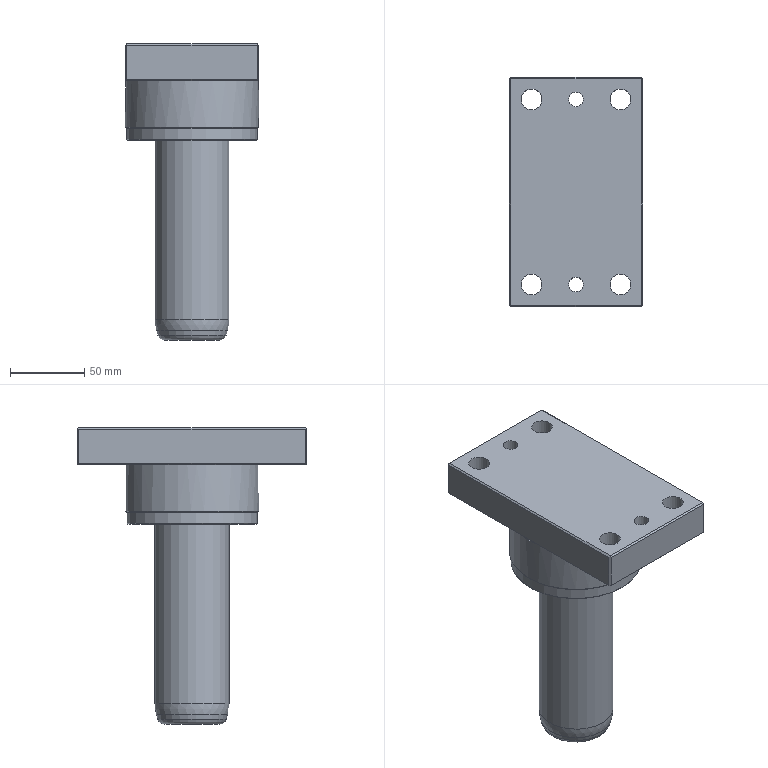Part | NX | features solid 2 | 1 solid | 46 faces | box 90 x 155 x 200 mm | volume 838352 mm3 | plane 26 | cylinder 13 | cone 5 | torus 2 | commonest cylinder face diameters 14 x4 50 x3 10 x2 12 x1 46 x1 88 x1
STEP:
#1=CARTESIAN_POINT('',(360.,263.5,441.));
#2=VERTEX_POINT('',#1);
#3=CARTESIAN_POINT('',(360.,334.084,441.));
#4=VERTEX_POINT('',#3);
#5=CARTESIAN_POINT('',(360.,262.5,441.));
#6=DIRECTION('',(0.,1.,0.));
#7=VECTOR('',#6,1000.);
#8=LINE('',#5,#7);
#9=EDGE_CURVE('',#2,#4,#8,.T.);
#10=ORIENTED_EDGE('',*,*,#9,.T.);
#11=CARTESIAN_POINT('',(360.,345.916,441.));
#12=VERTEX_POINT('',#11);
#13=CARTESIAN_POINT('',(360.,340.,440.));
#14=DIRECTION('',(1.,0.,0.));
#15=DIRECTION('',(0.,-1.,0.));
#16=AXIS2_PLACEMENT_3D('',#13,#14,#15);
#17=CIRCLE('',#16,6.);
#18=EDGE_CURVE('',#12,#4,#17,.T.);
#19=ORIENTED_EDGE('',*,*,#18,.F.);
#20=CARTESIAN_POINT('',(360.,416.5,441.));
#21=VERTEX_POINT('',#20);
#22=CARTESIAN_POINT('',(360.,262.5,441.));
#23=DIRECTION('',(0.,1.,0.));
#24=VECTOR('',#23,1000.);
#25=LINE('',#22,#24);
#26=EDGE_CURVE('',#12,#21,#25,.T.);
#27=ORIENTED_EDGE('',*,*,#26,.T.);
#28=CARTESIAN_POINT('',(360.,416.5,464.));
#29=VERTEX_POINT('',#28);
#30=CARTESIAN_POINT('',(360.,416.5,440.));
#31=DIRECTION('',(0.,0.,1.));
#32=VECTOR('',#31,1000.);
#33=LINE('',#30,#32);
#34=EDGE_CURVE('',#21,#29,#33,.T.);
#35=ORIENTED_EDGE('',*,*,#34,.T.);
#36=CARTESIAN_POINT('',(360.,263.5,464.));
#37=VERTEX_POINT('',#36);
#38=CARTESIAN_POINT('',(360.,262.5,464.));
#39=DIRECTION('',(0.,-1.,0.));
#40=VECTOR('',#39,1000.);
#41=LINE('',#38,#40);
#42=EDGE_CURVE('',#29,#37,#41,.T.);
#43=ORIENTED_EDGE('',*,*,#42,.T.);
#44=CARTESIAN_POINT('',(360.,263.5,440.));
#45=DIRECTION('',(0.,0.,-1.));
#46=VECTOR('',#45,1000.);
#47=LINE('',#44,#46);
#48=EDGE_CURVE('',#37,#2,#47,.T.);
#49=ORIENTED_EDGE('',*,*,#48,.T.);
#50=EDGE_LOOP('',(#10,#19,#27,#35,#43,#49));
#51=FACE_BOUND('',#50,.T.);
#52=CARTESIAN_POINT('',(360.,262.5,440.));
#53=DIRECTION('',(1.,0.,0.));
#54=DIRECTION('',(0.,-1.,0.));
#55=AXIS2_PLACEMENT_3D('',#52,#53,#54);
#56=PLANE('',#55);
#57=ADVANCED_FACE('',(#51),#56,.T.);
#58=CARTESIAN_POINT('',(359.,334.,440.));
#59=VERTEX_POINT('',#58);
#60=CARTESIAN_POINT('',(359.,330.566,440.));
#61=VERTEX_POINT('',#60);
#62=CARTESIAN_POINT('',(359.,417.5,440.));
#63=DIRECTION('',(0.,-1.,0.));
#64=VECTOR('',#63,1000.);
#65=LINE('',#62,#64);
#66=EDGE_CURVE('',#59,#61,#65,.T.);
#67=ORIENTED_EDGE('',*,*,#66,.F.);
#68=CARTESIAN_POINT('',(359.,340.,440.));
#69=DIRECTION('',(-0.7071,0.,0.7071));
#70=DIRECTION('',(-0.7071,0.,-0.7071));
#71=AXIS2_PLACEMENT_3D('',#68,#69,#70);
#72=ELLIPSE('',#71,8.485,6.);
#73=EDGE_CURVE('',#59,#4,#72,.T.);
#74=ORIENTED_EDGE('',*,*,#73,.T.);
#75=ORIENTED_EDGE('',*,*,#9,.F.);
#76=CARTESIAN_POINT('',(359.5,263.,440.5));
#77=VERTEX_POINT('',#76);
#78=CARTESIAN_POINT('',(359.667,263.167,440.667));
#79=DIRECTION('',(-0.5774,-0.5774,-0.5774));
#80=VECTOR('',#79,1000.);
#81=LINE('',#78,#80);
#82=EDGE_CURVE('',#2,#77,#81,.T.);
#83=ORIENTED_EDGE('',*,*,#82,.T.);
#84=CARTESIAN_POINT('',(359.,263.5,440.));
#85=VERTEX_POINT('',#84);
#86=CARTESIAN_POINT('',(360.,262.5,441.));
#87=DIRECTION('',(-0.5774,0.5774,-0.5774));
#88=VECTOR('',#87,1000.);
#89=LINE('',#86,#88);
#90=EDGE_CURVE('',#85,#77,#89,.F.);
#91=ORIENTED_EDGE('',*,*,#90,.F.);
#92=CARTESIAN_POINT('',(359.,417.5,440.));
#93=DIRECTION('',(0.,-1.,0.));
#94=VECTOR('',#93,1000.);
#95=LINE('',#92,#94);
#96=EDGE_CURVE('',#61,#85,#95,.T.);
#97=ORIENTED_EDGE('',*,*,#96,.F.);
#98=EDGE_LOOP('',(#67,#74,#75,#83,#91,#97));
#99=FACE_BOUND('',#98,.T.);
#100=CARTESIAN_POINT('',(360.,262.5,441.));
#101=DIRECTION('',(-0.7071,0.,0.7071));
#102=DIRECTION('',(-0.7071,0.,-0.7071));
#103=AXIS2_PLACEMENT_3D('',#100,#101,#102);
#104=PLANE('',#103);
#105=ADVANCED_FACE('',(#99),#104,.F.);
#106=ORIENTED_EDGE('',*,*,#26,.F.);
#107=CARTESIAN_POINT('',(359.,346.,440.));
#108=VERTEX_POINT('',#107);
#109=CARTESIAN_POINT('',(359.,340.,440.));
#110=DIRECTION('',(-0.7071,0.,0.7071));
#111=DIRECTION('',(-0.7071,0.,-0.7071));
#112=AXIS2_PLACEMENT_3D('',#109,#110,#111);
#113=ELLIPSE('',#112,8.485,6.);
#114=EDGE_CURVE('',#12,#108,#113,.T.);
#115=ORIENTED_EDGE('',*,*,#114,.T.);
#116=CARTESIAN_POINT('',(359.,349.434,440.));
#117=VERTEX_POINT('',#116);
#118=CARTESIAN_POINT('',(359.,417.5,440.));
#119=DIRECTION('',(0.,-1.,0.));
#120=VECTOR('',#119,1000.);
#121=LINE('',#118,#120);
#122=EDGE_CURVE('',#117,#108,#121,.T.);
#123=ORIENTED_EDGE('',*,*,#122,.F.);
#124=CARTESIAN_POINT('',(359.,416.5,440.));
#125=VERTEX_POINT('',#124);
#126=CARTESIAN_POINT('',(359.,417.5,440.));
#127=DIRECTION('',(0.,-1.,0.));
#128=VECTOR('',#127,1000.);
#129=LINE('',#126,#128);
#130=EDGE_CURVE('',#125,#117,#129,.T.);
#131=ORIENTED_EDGE('',*,*,#130,.F.);
#132=CARTESIAN_POINT('',(359.5,417.,440.5));
#133=VERTEX_POINT('',#132);
#134=CARTESIAN_POINT('',(360.,417.5,441.));
#135=DIRECTION('',(-0.5774,-0.5774,-0.5774));
#136=VECTOR('',#135,1000.);
#137=LINE('',#134,#136);
#138=EDGE_CURVE('',#125,#133,#137,.F.);
#139=ORIENTED_EDGE('',*,*,#138,.T.);
#140=CARTESIAN_POINT('',(411.333,365.167,492.333));
#141=DIRECTION('',(0.5774,-0.5774,0.5774));
#142=VECTOR('',#141,1000.);
#143=LINE('',#140,#142);
#144=EDGE_CURVE('',#133,#21,#143,.T.);
#145=ORIENTED_EDGE('',*,*,#144,.T.);
#146=EDGE_LOOP('',(#106,#115,#123,#131,#139,#145));
#147=FACE_BOUND('',#146,.T.);
#148=CARTESIAN_POINT('',(360.,262.5,441.));
#149=DIRECTION('',(-0.7071,0.,0.7071));
#150=DIRECTION('',(-0.7071,0.,-0.7071));
#151=AXIS2_PLACEMENT_3D('',#148,#149,#150);
#152=PLANE('',#151);
#153=ADVANCED_FACE('',(#147),#152,.F.);
#154=CARTESIAN_POINT('',(359.598,334.,440.));
#155=VERTEX_POINT('',#154);
#156=CARTESIAN_POINT('',(360.,334.,440.));
#157=DIRECTION('',(-1.,0.,0.));
#158=VECTOR('',#157,1000.);
#159=LINE('',#156,#158);
#160=EDGE_CURVE('',#59,#155,#159,.F.);
#161=ORIENTED_EDGE('',*,*,#160,.F.);
#162=ORIENTED_EDGE('',*,*,#66,.T.);
#163=CARTESIAN_POINT('',(315.,340.,440.));
#164=DIRECTION('',(0.,0.,-1.));
#165=DIRECTION('',(0.,-1.,0.));
#166=AXIS2_PLACEMENT_3D('',#163,#164,#165);
#167=CIRCLE('',#166,45.);
#168=EDGE_CURVE('',#155,#61,#167,.T.);
#169=ORIENTED_EDGE('',*,*,#168,.F.);
#170=EDGE_LOOP('',(#161,#162,#169));
#171=FACE_BOUND('',#170,.T.);
#172=CARTESIAN_POINT('',(315.,340.,440.));
#173=DIRECTION('',(0.,0.,-1.));
#174=DIRECTION('',(0.,-1.,0.));
#175=AXIS2_PLACEMENT_3D('',#172,#173,#174);
#176=PLANE('',#175);
#177=ADVANCED_FACE('',(#171),#176,.F.);
#178=CARTESIAN_POINT('',(359.598,346.,440.));
#179=VERTEX_POINT('',#178);
#180=CARTESIAN_POINT('',(360.,346.,440.));
#181=DIRECTION('',(-1.,0.,0.));
#182=VECTOR('',#181,1000.);
#183=LINE('',#180,#182);
#184=EDGE_CURVE('',#179,#108,#183,.T.);
#185=ORIENTED_EDGE('',*,*,#184,.F.);
#186=CARTESIAN_POINT('',(315.,340.,440.));
#187=DIRECTION('',(0.,0.,-1.));
#188=DIRECTION('',(0.,-1.,0.));
#189=AXIS2_PLACEMENT_3D('',#186,#187,#188);
#190=CIRCLE('',#189,45.);
#191=EDGE_CURVE('',#117,#179,#190,.T.);
#192=ORIENTED_EDGE('',*,*,#191,.F.);
#193=ORIENTED_EDGE('',*,*,#122,.T.);
#194=EDGE_LOOP('',(#185,#192,#193));
#195=FACE_BOUND('',#194,.T.);
#196=CARTESIAN_POINT('',(315.,340.,440.));
#197=DIRECTION('',(0.,0.,-1.));
#198=DIRECTION('',(0.,-1.,0.));
#199=AXIS2_PLACEMENT_3D('',#196,#197,#198);
#200=PLANE('',#199);
#201=ADVANCED_FACE('',(#195),#200,.F.);
#202=CARTESIAN_POINT('',(315.,295.,408.625));
#203=VERTEX_POINT('',#202);
#204=CARTESIAN_POINT('',(315.,340.,408.625));
#205=DIRECTION('',(0.,0.,-1.));
#206=DIRECTION('',(0.,-1.,0.));
#207=AXIS2_PLACEMENT_3D('',#204,#205,#206);
#208=CIRCLE('',#207,45.);
#209=EDGE_CURVE('',#203,#203,#208,.F.);
#210=ORIENTED_EDGE('',*,*,#209,.T.);
#211=EDGE_LOOP('',(#210));
#212=FACE_BOUND('',#211,.T.);
#213=CARTESIAN_POINT('',(359.598,334.,440.));
#214=CARTESIAN_POINT('',(359.598,334.,438.413));
#215=CARTESIAN_POINT('',(359.8,335.296,435.31));
#216=CARTESIAN_POINT('',(360.1,340.001,433.346));
#217=CARTESIAN_POINT('',(359.8,344.699,435.306));
#218=CARTESIAN_POINT('',(359.598,346.,438.413));
#219=CARTESIAN_POINT('',(359.598,346.,440.));
#220=B_SPLINE_CURVE_WITH_KNOTS('',3,(#213,#214,#215,#216,#217,#218,#219),.UNSPECIFIED.,.F.,.F.,(4,1,1,1,4),(0.,0.004692,0.009383,0.01408,0.01877),.UNSPECIFIED.);
#221=EDGE_CURVE('',#155,#179,#220,.T.);
#222=ORIENTED_EDGE('',*,*,#221,.F.);
#223=ORIENTED_EDGE('',*,*,#168,.T.);
#224=CARTESIAN_POINT('',(271.,330.566,440.));
#225=VERTEX_POINT('',#224);
#226=CARTESIAN_POINT('',(315.,340.,440.));
#227=DIRECTION('',(0.,0.,-1.));
#228=DIRECTION('',(0.,-1.,0.));
#229=AXIS2_PLACEMENT_3D('',#226,#227,#228);
#230=CIRCLE('',#229,45.);
#231=EDGE_CURVE('',#61,#225,#230,.T.);
#232=ORIENTED_EDGE('',*,*,#231,.T.);
#233=CARTESIAN_POINT('',(271.,349.434,440.));
#234=VERTEX_POINT('',#233);
#235=CARTESIAN_POINT('',(315.,340.,440.));
#236=DIRECTION('',(0.,0.,-1.));
#237=DIRECTION('',(0.,-1.,0.));
#238=AXIS2_PLACEMENT_3D('',#235,#236,#237);
#239=CIRCLE('',#238,45.);
#240=EDGE_CURVE('',#225,#234,#239,.T.);
#241=ORIENTED_EDGE('',*,*,#240,.T.);
#242=CARTESIAN_POINT('',(315.,340.,440.));
#243=DIRECTION('',(0.,0.,-1.));
#244=DIRECTION('',(0.,-1.,0.));
#245=AXIS2_PLACEMENT_3D('',#242,#243,#244);
#246=CIRCLE('',#245,45.);
#247=EDGE_CURVE('',#234,#117,#246,.T.);
#248=ORIENTED_EDGE('',*,*,#247,.T.);
#249=ORIENTED_EDGE('',*,*,#191,.T.);
#250=EDGE_LOOP('',(#222,#223,#232,#241,#248,#249));
#251=FACE_BOUND('',#250,.T.);
#252=CARTESIAN_POINT('',(315.,340.,408.125));
#253=DIRECTION('',(0.,0.,1.));
#254=DIRECTION('',(0.,1.,0.));
#255=AXIS2_PLACEMENT_3D('',#252,#253,#254);
#256=CYLINDRICAL_SURFACE('',#255,45.);
#257=ADVANCED_FACE('',(#212,#251),#256,.T.);
#258=CARTESIAN_POINT('',(315.,365.,426.5));
#259=VERTEX_POINT('',#258);
#260=CARTESIAN_POINT('',(315.,340.,426.5));
#261=DIRECTION('',(0.,0.,-1.));
#262=DIRECTION('',(0.,1.,0.));
#263=AXIS2_PLACEMENT_3D('',#260,#261,#262);
#264=CIRCLE('',#263,25.);
#265=EDGE_CURVE('',#259,#259,#264,.F.);
#266=ORIENTED_EDGE('',*,*,#265,.F.);
#267=EDGE_LOOP('',(#266));
#268=FACE_BOUND('',#267,.T.);
#269=CARTESIAN_POINT('',(339.316,345.809,438.5));
#270=VERTEX_POINT('',#269);
#271=CARTESIAN_POINT('',(339.316,334.191,438.5));
#272=VERTEX_POINT('',#271);
#273=CARTESIAN_POINT('',(315.,340.,438.5));
#274=DIRECTION('',(0.,0.,-1.));
#275=DIRECTION('',(0.,-1.,0.));
#276=AXIS2_PLACEMENT_3D('',#273,#274,#275);
#277=CIRCLE('',#276,25.);
#278=EDGE_CURVE('',#270,#272,#277,.F.);
#279=ORIENTED_EDGE('',*,*,#278,.T.);
#280=CARTESIAN_POINT('',(339.316,334.191,438.5));
#281=CARTESIAN_POINT('',(339.395,334.522,437.217));
#282=CARTESIAN_POINT('',(339.758,336.04,434.912));
#283=CARTESIAN_POINT('',(340.121,340.007,433.543));
#284=CARTESIAN_POINT('',(339.758,343.961,434.917));
#285=CARTESIAN_POINT('',(339.395,345.477,437.213));
#286=CARTESIAN_POINT('',(339.316,345.809,438.5));
#287=B_SPLINE_CURVE_WITH_KNOTS('',3,(#280,#281,#282,#283,#284,#285,#286),.UNSPECIFIED.,.F.,.F.,(4,1,1,1,4),(0.02975,0.0337,0.03765,0.04161,0.04556),.UNSPECIFIED.);
#288=EDGE_CURVE('',#272,#270,#287,.T.);
#289=ORIENTED_EDGE('',*,*,#288,.T.);
#290=EDGE_LOOP('',(#279,#289));
#291=FACE_BOUND('',#290,.T.);
#292=CARTESIAN_POINT('',(315.,340.,400.));
#293=DIRECTION('',(0.,0.,1.));
#294=DIRECTION('',(0.,1.,0.));
#295=AXIS2_PLACEMENT_3D('',#292,#293,#294);
#296=CYLINDRICAL_SURFACE('',#295,25.);
#297=ADVANCED_FACE('',(#268,#291),#296,.F.);
#298=CARTESIAN_POINT('',(315.,407.5,465.));
#299=VERTEX_POINT('',#298);
#300=CARTESIAN_POINT('',(315.,402.5,465.));
#301=DIRECTION('',(0.,0.,1.));
#302=DIRECTION('',(0.,1.,0.));
#303=AXIS2_PLACEMENT_3D('',#300,#301,#302);
#304=CIRCLE('',#303,5.);
#305=EDGE_CURVE('',#299,#299,#304,.T.);
#306=ORIENTED_EDGE('',*,*,#305,.F.);
#307=EDGE_LOOP('',(#306));
#308=FACE_BOUND('',#307,.T.);
#309=CARTESIAN_POINT('',(345.,409.5,465.));
#310=VERTEX_POINT('',#309);
#311=CARTESIAN_POINT('',(345.,402.5,465.));
#312=DIRECTION('',(0.,0.,-1.));
#313=DIRECTION('',(0.,1.,0.));
#314=AXIS2_PLACEMENT_3D('',#311,#312,#313);
#315=CIRCLE('',#314,7.);
#316=EDGE_CURVE('',#310,#310,#315,.T.);
#317=ORIENTED_EDGE('',*,*,#316,.T.);
#318=EDGE_LOOP('',(#317));
#319=FACE_BOUND('',#318,.T.);
#320=CARTESIAN_POINT('',(345.,270.5,465.));
#321=VERTEX_POINT('',#320);
#322=CARTESIAN_POINT('',(345.,277.5,465.));
#323=DIRECTION('',(0.,0.,1.));
#324=DIRECTION('',(0.,-1.,0.));
#325=AXIS2_PLACEMENT_3D('',#322,#323,#324);
#326=CIRCLE('',#325,7.);
#327=EDGE_CURVE('',#321,#321,#326,.T.);
#328=ORIENTED_EDGE('',*,*,#327,.F.);
#329=EDGE_LOOP('',(#328));
#330=FACE_BOUND('',#329,.T.);
#331=CARTESIAN_POINT('',(271.,416.5,465.));
#332=VERTEX_POINT('',#331);
#333=CARTESIAN_POINT('',(271.,263.5,465.));
#334=VERTEX_POINT('',#333);
#335=CARTESIAN_POINT('',(271.,262.5,465.));
#336=DIRECTION('',(0.,-1.,0.));
#337=VECTOR('',#336,1000.);
#338=LINE('',#335,#337);
#339=EDGE_CURVE('',#332,#334,#338,.T.);
#340=ORIENTED_EDGE('',*,*,#339,.T.);
#341=CARTESIAN_POINT('',(359.,263.5,465.));
#342=VERTEX_POINT('',#341);
#343=CARTESIAN_POINT('',(360.,263.5,465.));
#344=DIRECTION('',(1.,0.,0.));
#345=VECTOR('',#344,1000.);
#346=LINE('',#343,#345);
#347=EDGE_CURVE('',#334,#342,#346,.T.);
#348=ORIENTED_EDGE('',*,*,#347,.T.);
#349=CARTESIAN_POINT('',(359.,416.5,465.));
#350=VERTEX_POINT('',#349);
#351=CARTESIAN_POINT('',(359.,417.5,465.));
#352=DIRECTION('',(0.,1.,0.));
#353=VECTOR('',#352,1000.);
#354=LINE('',#351,#353);
#355=EDGE_CURVE('',#342,#350,#354,.T.);
#356=ORIENTED_EDGE('',*,*,#355,.T.);
#357=CARTESIAN_POINT('',(270.,416.5,465.));
#358=DIRECTION('',(-1.,0.,0.));
#359=VECTOR('',#358,1000.);
#360=LINE('',#357,#359);
#361=EDGE_CURVE('',#350,#332,#360,.T.);
#362=ORIENTED_EDGE('',*,*,#361,.T.);
#363=EDGE_LOOP('',(#340,#348,#356,#362));
#364=FACE_BOUND('',#363,.T.);
#365=CARTESIAN_POINT('',(285.,270.5,465.));
#366=VERTEX_POINT('',#365);
#367=CARTESIAN_POINT('',(285.,277.5,465.));
#368=DIRECTION('',(0.,0.,-1.));
#369=DIRECTION('',(0.,-1.,0.));
#370=AXIS2_PLACEMENT_3D('',#367,#368,#369);
#371=CIRCLE('',#370,7.);
#372=EDGE_CURVE('',#366,#366,#371,.T.);
#373=ORIENTED_EDGE('',*,*,#372,.T.);
#374=EDGE_LOOP('',(#373));
#375=FACE_BOUND('',#374,.T.);
#376=CARTESIAN_POINT('',(285.,409.5,465.));
#377=VERTEX_POINT('',#376);
#378=CARTESIAN_POINT('',(285.,402.5,465.));
#379=DIRECTION('',(0.,0.,1.));
#380=DIRECTION('',(0.,1.,0.));
#381=AXIS2_PLACEMENT_3D('',#378,#379,#380);
#382=CIRCLE('',#381,7.);
#383=EDGE_CURVE('',#377,#377,#382,.T.);
#384=ORIENTED_EDGE('',*,*,#383,.F.);
#385=EDGE_LOOP('',(#384));
#386=FACE_BOUND('',#385,.T.);
#387=CARTESIAN_POINT('',(315.,272.5,465.));
#388=VERTEX_POINT('',#387);
#389=CARTESIAN_POINT('',(315.,277.5,465.));
#390=DIRECTION('',(0.,0.,-1.));
#391=DIRECTION('',(0.,-1.,0.));
#392=AXIS2_PLACEMENT_3D('',#389,#390,#391);
#393=CIRCLE('',#392,5.);
#394=EDGE_CURVE('',#388,#388,#393,.T.);
#395=ORIENTED_EDGE('',*,*,#394,.T.);
#396=EDGE_LOOP('',(#395));
#397=FACE_BOUND('',#396,.T.);
#398=CARTESIAN_POINT('',(360.,417.5,465.));
#399=DIRECTION('',(0.,0.,-1.));
#400=DIRECTION('',(0.,-1.,0.));
#401=AXIS2_PLACEMENT_3D('',#398,#399,#400);
#402=PLANE('',#401);
#403=ADVANCED_FACE('',(#308,#319,#330,#364,#375,#386,#397),#402,.F.);
#404=CARTESIAN_POINT('',(285.,270.5,440.));
#405=VERTEX_POINT('',#404);
#406=CARTESIAN_POINT('',(285.,277.5,440.));
#407=DIRECTION('',(0.,0.,-1.));
#408=DIRECTION('',(0.,-1.,0.));
#409=AXIS2_PLACEMENT_3D('',#406,#407,#408);
#410=CIRCLE('',#409,7.);
#411=EDGE_CURVE('',#405,#405,#410,.F.);
#412=ORIENTED_EDGE('',*,*,#411,.T.);
#413=EDGE_LOOP('',(#412));
#414=FACE_BOUND('',#413,.T.);
#415=ORIENTED_EDGE('',*,*,#231,.F.);
#416=ORIENTED_EDGE('',*,*,#96,.T.);
#417=CARTESIAN_POINT('',(271.,263.5,440.));
#418=VERTEX_POINT('',#417);
#419=CARTESIAN_POINT('',(360.,263.5,440.));
#420=DIRECTION('',(-1.,0.,0.));
#421=VECTOR('',#420,1000.);
#422=LINE('',#419,#421);
#423=EDGE_CURVE('',#85,#418,#422,.T.);
#424=ORIENTED_EDGE('',*,*,#423,.T.);
#425=CARTESIAN_POINT('',(271.,417.5,440.));
#426=DIRECTION('',(0.,1.,0.));
#427=VECTOR('',#426,1000.);
#428=LINE('',#425,#427);
#429=EDGE_CURVE('',#418,#225,#428,.T.);
#430=ORIENTED_EDGE('',*,*,#429,.T.);
#431=EDGE_LOOP('',(#415,#416,#424,#430));
#432=FACE_BOUND('',#431,.T.);
#433=CARTESIAN_POINT('',(345.,270.5,440.));
#434=VERTEX_POINT('',#433);
#435=CARTESIAN_POINT('',(345.,277.5,440.));
#436=DIRECTION('',(0.,0.,-1.));
#437=DIRECTION('',(0.,-1.,0.));
#438=AXIS2_PLACEMENT_3D('',#435,#436,#437);
#439=CIRCLE('',#438,7.);
#440=EDGE_CURVE('',#434,#434,#439,.T.);
#441=ORIENTED_EDGE('',*,*,#440,.F.);
#442=EDGE_LOOP('',(#441));
#443=FACE_BOUND('',#442,.T.);
#444=CARTESIAN_POINT('',(315.,272.5,440.));
#445=VERTEX_POINT('',#444);
#446=CARTESIAN_POINT('',(315.,277.5,440.));
#447=DIRECTION('',(0.,0.,-1.));
#448=DIRECTION('',(0.,-1.,0.));
#449=AXIS2_PLACEMENT_3D('',#446,#447,#448);
#450=CIRCLE('',#449,5.);
#451=EDGE_CURVE('',#445,#445,#450,.T.);
#452=ORIENTED_EDGE('',*,*,#451,.F.);
#453=EDGE_LOOP('',(#452));
#454=FACE_BOUND('',#453,.T.);
#455=CARTESIAN_POINT('',(360.,417.5,440.));
#456=DIRECTION('',(0.,0.,-1.));
#457=DIRECTION('',(0.,-1.,0.));
#458=AXIS2_PLACEMENT_3D('',#455,#456,#457);
#459=PLANE('',#458);
#460=ADVANCED_FACE('',(#414,#432,#443,#454),#459,.T.);
#461=CARTESIAN_POINT('',(315.,407.5,440.));
#462=VERTEX_POINT('',#461);
#463=CARTESIAN_POINT('',(315.,402.5,440.));
#464=DIRECTION('',(0.,0.,1.));
#465=DIRECTION('',(0.,1.,0.));
#466=AXIS2_PLACEMENT_3D('',#463,#464,#465);
#467=CIRCLE('',#466,5.);
#468=EDGE_CURVE('',#462,#462,#467,.T.);
#469=ORIENTED_EDGE('',*,*,#468,.T.);
#470=EDGE_LOOP('',(#469));
#471=FACE_BOUND('',#470,.T.);
#472=CARTESIAN_POINT('',(285.,395.5,440.));
#473=VERTEX_POINT('',#472);
#474=CARTESIAN_POINT('',(285.,402.5,440.));
#475=DIRECTION('',(0.,0.,-1.));
#476=DIRECTION('',(0.,-1.,0.));
#477=AXIS2_PLACEMENT_3D('',#474,#475,#476);
#478=CIRCLE('',#477,7.);
#479=EDGE_CURVE('',#473,#473,#478,.T.);
#480=ORIENTED_EDGE('',*,*,#479,.F.);
#481=EDGE_LOOP('',(#480));
#482=FACE_BOUND('',#481,.T.);
#483=ORIENTED_EDGE('',*,*,#247,.F.);
#484=CARTESIAN_POINT('',(271.,416.5,440.));
#485=VERTEX_POINT('',#484);
#486=CARTESIAN_POINT('',(271.,417.5,440.));
#487=DIRECTION('',(0.,1.,0.));
#488=VECTOR('',#487,1000.);
#489=LINE('',#486,#488);
#490=EDGE_CURVE('',#234,#485,#489,.T.);
#491=ORIENTED_EDGE('',*,*,#490,.T.);
#492=CARTESIAN_POINT('',(360.,416.5,440.));
#493=DIRECTION('',(1.,0.,0.));
#494=VECTOR('',#493,1000.);
#495=LINE('',#492,#494);
#496=EDGE_CURVE('',#485,#125,#495,.T.);
#497=ORIENTED_EDGE('',*,*,#496,.T.);
#498=ORIENTED_EDGE('',*,*,#130,.T.);
#499=EDGE_LOOP('',(#483,#491,#497,#498));
#500=FACE_BOUND('',#499,.T.);
#501=CARTESIAN_POINT('',(345.,395.5,440.));
#502=VERTEX_POINT('',#501);
#503=CARTESIAN_POINT('',(345.,402.5,440.));
#504=DIRECTION('',(0.,0.,-1.));
#505=DIRECTION('',(0.,-1.,0.));
#506=AXIS2_PLACEMENT_3D('',#503,#504,#505);
#507=CIRCLE('',#506,7.);
#508=EDGE_CURVE('',#502,#502,#507,.F.);
#509=ORIENTED_EDGE('',*,*,#508,.T.);
#510=EDGE_LOOP('',(#509));
#511=FACE_BOUND('',#510,.T.);
#512=CARTESIAN_POINT('',(360.,417.5,440.));
#513=DIRECTION('',(0.,0.,-1.));
#514=DIRECTION('',(0.,-1.,0.));
#515=AXIS2_PLACEMENT_3D('',#512,#513,#514);
#516=PLANE('',#515);
#517=ADVANCED_FACE('',(#471,#482,#500,#511),#516,.T.);
#518=CARTESIAN_POINT('',(315.,296.5,400.));
#519=VERTEX_POINT('',#518);
#520=CARTESIAN_POINT('',(315.,340.,400.));
#521=DIRECTION('',(0.,0.,-1.));
#522=DIRECTION('',(0.,-1.,0.));
#523=AXIS2_PLACEMENT_3D('',#520,#521,#522);
#524=CIRCLE('',#523,43.5);
#525=EDGE_CURVE('',#519,#519,#524,.T.);
#526=ORIENTED_EDGE('',*,*,#525,.T.);
#527=EDGE_LOOP('',(#526));
#528=FACE_BOUND('',#527,.T.);
#529=CARTESIAN_POINT('',(315.,315.,400.));
#530=VERTEX_POINT('',#529);
#531=CARTESIAN_POINT('',(315.,340.,400.));
#532=DIRECTION('',(0.,0.,-1.));
#533=DIRECTION('',(0.,-1.,0.));
#534=AXIS2_PLACEMENT_3D('',#531,#532,#533);
#535=CIRCLE('',#534,25.);
#536=EDGE_CURVE('',#530,#530,#535,.T.);
#537=ORIENTED_EDGE('',*,*,#536,.F.);
#538=EDGE_LOOP('',(#537));
#539=FACE_BOUND('',#538,.T.);
#540=CARTESIAN_POINT('',(315.,340.,400.));
#541=DIRECTION('',(0.,0.,-1.));
#542=DIRECTION('',(0.,-1.,0.));
#543=AXIS2_PLACEMENT_3D('',#540,#541,#542);
#544=PLANE('',#543);
#545=ADVANCED_FACE('',(#528,#539),#544,.T.);
#546=CARTESIAN_POINT('',(315.,295.5,408.125));
#547=VERTEX_POINT('',#546);
#548=CARTESIAN_POINT('',(315.,340.,408.125));
#549=DIRECTION('',(0.,0.,-1.));
#550=DIRECTION('',(0.,-1.,0.));
#551=AXIS2_PLACEMENT_3D('',#548,#549,#550);
#552=CIRCLE('',#551,44.5);
#553=EDGE_CURVE('',#547,#547,#552,.T.);
#554=ORIENTED_EDGE('',*,*,#553,.T.);
#555=EDGE_LOOP('',(#554));
#556=FACE_BOUND('',#555,.T.);
#557=CARTESIAN_POINT('',(315.,296.,408.125));
#558=VERTEX_POINT('',#557);
#559=CARTESIAN_POINT('',(315.,340.,408.125));
#560=DIRECTION('',(0.,0.,-1.));
#561=DIRECTION('',(0.,-1.,0.));
#562=AXIS2_PLACEMENT_3D('',#559,#560,#561);
#563=CIRCLE('',#562,44.);
#564=EDGE_CURVE('',#558,#558,#563,.T.);
#565=ORIENTED_EDGE('',*,*,#564,.F.);
#566=EDGE_LOOP('',(#565));
#567=FACE_BOUND('',#566,.T.);
#568=CARTESIAN_POINT('',(315.,340.,408.125));
#569=DIRECTION('',(0.,0.,-1.));
#570=DIRECTION('',(0.,-1.,0.));
#571=AXIS2_PLACEMENT_3D('',#568,#569,#570);
#572=PLANE('',#571);
#573=ADVANCED_FACE('',(#556,#567),#572,.T.);
#574=CARTESIAN_POINT('',(271.,417.5,464.));
#575=VERTEX_POINT('',#574);
#576=CARTESIAN_POINT('',(359.,417.5,464.));
#577=VERTEX_POINT('',#576);
#578=CARTESIAN_POINT('',(360.,417.5,464.));
#579=DIRECTION('',(1.,0.,0.));
#580=VECTOR('',#579,1000.);
#581=LINE('',#578,#580);
#582=EDGE_CURVE('',#575,#577,#581,.T.);
#583=ORIENTED_EDGE('',*,*,#582,.T.);
#584=CARTESIAN_POINT('',(359.,417.5,441.));
#585=VERTEX_POINT('',#584);
#586=CARTESIAN_POINT('',(359.,417.5,440.));
#587=DIRECTION('',(0.,0.,-1.));
#588=VECTOR('',#587,1000.);
#589=LINE('',#586,#588);
#590=EDGE_CURVE('',#577,#585,#589,.T.);
#591=ORIENTED_EDGE('',*,*,#590,.T.);
#592=CARTESIAN_POINT('',(271.,417.5,441.));
#593=VERTEX_POINT('',#592);
#594=CARTESIAN_POINT('',(360.,417.5,441.));
#595=DIRECTION('',(-1.,0.,0.));
#596=VECTOR('',#595,1000.);
#597=LINE('',#594,#596);
#598=EDGE_CURVE('',#585,#593,#597,.T.);
#599=ORIENTED_EDGE('',*,*,#598,.T.);
#600=CARTESIAN_POINT('',(271.,417.5,440.));
#601=DIRECTION('',(0.,0.,1.));
#602=VECTOR('',#601,1000.);
#603=LINE('',#600,#602);
#604=EDGE_CURVE('',#593,#575,#603,.T.);
#605=ORIENTED_EDGE('',*,*,#604,.T.);
#606=EDGE_LOOP('',(#583,#591,#599,#605));
#607=FACE_BOUND('',#606,.T.);
#608=CARTESIAN_POINT('',(360.,417.5,440.));
#609=DIRECTION('',(0.,1.,0.));
#610=DIRECTION('',(0.,0.,-1.));
#611=AXIS2_PLACEMENT_3D('',#608,#609,#610);
#612=PLANE('',#611);
#613=ADVANCED_FACE('',(#607),#612,.T.);
#614=CARTESIAN_POINT('',(270.,263.5,464.));
#615=VERTEX_POINT('',#614);
#616=CARTESIAN_POINT('',(270.,416.5,464.));
#617=VERTEX_POINT('',#616);
#618=CARTESIAN_POINT('',(270.,417.5,464.));
#619=DIRECTION('',(0.,1.,0.));
#620=VECTOR('',#619,1000.);
#621=LINE('',#618,#620);
#622=EDGE_CURVE('',#615,#617,#621,.T.);
#623=ORIENTED_EDGE('',*,*,#622,.T.);
#624=CARTESIAN_POINT('',(270.,416.5,441.));
#625=VERTEX_POINT('',#624);
#626=CARTESIAN_POINT('',(270.,416.5,440.));
#627=DIRECTION('',(0.,0.,-1.));
#628=VECTOR('',#627,1000.);
#629=LINE('',#626,#628);
#630=EDGE_CURVE('',#617,#625,#629,.T.);
#631=ORIENTED_EDGE('',*,*,#630,.T.);
#632=CARTESIAN_POINT('',(270.,263.5,441.));
#633=VERTEX_POINT('',#632);
#634=CARTESIAN_POINT('',(270.,417.5,441.));
#635=DIRECTION('',(0.,-1.,0.));
#636=VECTOR('',#635,1000.);
#637=LINE('',#634,#636);
#638=EDGE_CURVE('',#625,#633,#637,.T.);
#639=ORIENTED_EDGE('',*,*,#638,.T.);
#640=CARTESIAN_POINT('',(270.,263.5,440.));
#641=DIRECTION('',(0.,0.,1.));
#642=VECTOR('',#641,1000.);
#643=LINE('',#640,#642);
#644=EDGE_CURVE('',#633,#615,#643,.T.);
#645=ORIENTED_EDGE('',*,*,#644,.T.);
#646=EDGE_LOOP('',(#623,#631,#639,#645));
#647=FACE_BOUND('',#646,.T.);
#648=CARTESIAN_POINT('',(270.,417.5,440.));
#649=DIRECTION('',(-1.,0.,0.));
#650=DIRECTION('',(0.,1.,0.));
#651=AXIS2_PLACEMENT_3D('',#648,#649,#650);
#652=PLANE('',#651);
#653=ADVANCED_FACE('',(#647),#652,.T.);
#654=CARTESIAN_POINT('',(271.,262.5,441.));
#655=VERTEX_POINT('',#654);
#656=CARTESIAN_POINT('',(359.,262.5,441.));
#657=VERTEX_POINT('',#656);
#658=CARTESIAN_POINT('',(270.,262.5,441.));
#659=DIRECTION('',(1.,0.,0.));
#660=VECTOR('',#659,1000.);
#661=LINE('',#658,#660);
#662=EDGE_CURVE('',#655,#657,#661,.T.);
#663=ORIENTED_EDGE('',*,*,#662,.T.);
#664=CARTESIAN_POINT('',(359.,262.5,464.));
#665=VERTEX_POINT('',#664);
#666=CARTESIAN_POINT('',(359.,262.5,440.));
#667=DIRECTION('',(0.,0.,1.));
#668=VECTOR('',#667,1000.);
#669=LINE('',#666,#668);
#670=EDGE_CURVE('',#657,#665,#669,.T.);
#671=ORIENTED_EDGE('',*,*,#670,.T.);
#672=CARTESIAN_POINT('',(271.,262.5,464.));
#673=VERTEX_POINT('',#672);
#674=CARTESIAN_POINT('',(270.,262.5,464.));
#675=DIRECTION('',(-1.,0.,0.));
#676=VECTOR('',#675,1000.);
#677=LINE('',#674,#676);
#678=EDGE_CURVE('',#665,#673,#677,.T.);
#679=ORIENTED_EDGE('',*,*,#678,.T.);
#680=CARTESIAN_POINT('',(271.,262.5,440.));
#681=DIRECTION('',(0.,0.,-1.));
#682=VECTOR('',#681,1000.);
#683=LINE('',#680,#682);
#684=EDGE_CURVE('',#673,#655,#683,.T.);
#685=ORIENTED_EDGE('',*,*,#684,.T.);
#686=EDGE_LOOP('',(#663,#671,#679,#685));
#687=FACE_BOUND('',#686,.T.);
#688=CARTESIAN_POINT('',(270.,262.5,440.));
#689=DIRECTION('',(0.,-1.,0.));
#690=DIRECTION('',(-1.,0.,0.));
#691=AXIS2_PLACEMENT_3D('',#688,#689,#690);
#692=PLANE('',#691);
#693=ADVANCED_FACE('',(#687),#692,.T.);
#694=CARTESIAN_POINT('',(359.5,417.,464.5));
#695=VERTEX_POINT('',#694);
#696=CARTESIAN_POINT('',(359.333,416.833,464.667));
#697=DIRECTION('',(0.5774,0.5774,-0.5774));
#698=VECTOR('',#697,1000.);
#699=LINE('',#696,#698);
#700=EDGE_CURVE('',#695,#350,#699,.F.);
#701=ORIENTED_EDGE('',*,*,#700,.F.);
#702=CARTESIAN_POINT('',(360.,416.5,465.));
#703=DIRECTION('',(0.5774,-0.5774,0.5774));
#704=VECTOR('',#703,1000.);
#705=LINE('',#702,#704);
#706=EDGE_CURVE('',#695,#577,#705,.F.);
#707=ORIENTED_EDGE('',*,*,#706,.T.);
#708=ORIENTED_EDGE('',*,*,#582,.F.);
#709=CARTESIAN_POINT('',(270.5,417.,464.5));
#710=VERTEX_POINT('',#709);
#711=CARTESIAN_POINT('',(300.,446.5,435.));
#712=DIRECTION('',(0.5774,0.5774,-0.5774));
#713=VECTOR('',#712,1000.);
#714=LINE('',#711,#713);
#715=EDGE_CURVE('',#575,#710,#714,.F.);
#716=ORIENTED_EDGE('',*,*,#715,.T.);
#717=CARTESIAN_POINT('',(270.667,416.833,464.667));
#718=DIRECTION('',(-0.5774,0.5774,-0.5774));
#719=VECTOR('',#718,1000.);
#720=LINE('',#717,#719);
#721=EDGE_CURVE('',#332,#710,#720,.T.);
#722=ORIENTED_EDGE('',*,*,#721,.F.);
#723=ORIENTED_EDGE('',*,*,#361,.F.);
#724=EDGE_LOOP('',(#701,#707,#708,#716,#722,#723));
#725=FACE_BOUND('',#724,.T.);
#726=CARTESIAN_POINT('',(360.,416.5,465.));
#727=DIRECTION('',(0.,0.7071,0.7071));
#728=DIRECTION('',(0.,0.7071,-0.7071));
#729=AXIS2_PLACEMENT_3D('',#726,#727,#728);
#730=PLANE('',#729);
#731=ADVANCED_FACE('',(#725),#730,.T.);
#732=ORIENTED_EDGE('',*,*,#721,.T.);
#733=CARTESIAN_POINT('',(271.,417.5,465.));
#734=DIRECTION('',(0.5774,0.5774,0.5774));
#735=VECTOR('',#734,1000.);
#736=LINE('',#733,#735);
#737=EDGE_CURVE('',#710,#617,#736,.F.);
#738=ORIENTED_EDGE('',*,*,#737,.T.);
#739=ORIENTED_EDGE('',*,*,#622,.F.);
#740=CARTESIAN_POINT('',(270.5,263.,464.5));
#741=VERTEX_POINT('',#740);
#742=CARTESIAN_POINT('',(219.333,314.167,413.333));
#743=DIRECTION('',(-0.5774,0.5774,-0.5774));
#744=VECTOR('',#743,1000.);
#745=LINE('',#742,#744);
#746=EDGE_CURVE('',#615,#741,#745,.F.);
#747=ORIENTED_EDGE('',*,*,#746,.T.);
#748=CARTESIAN_POINT('',(322.333,314.833,516.333));
#749=DIRECTION('',(0.5774,0.5774,0.5774));
#750=VECTOR('',#749,1000.);
#751=LINE('',#748,#750);
#752=EDGE_CURVE('',#334,#741,#751,.F.);
#753=ORIENTED_EDGE('',*,*,#752,.F.);
#754=ORIENTED_EDGE('',*,*,#339,.F.);
#755=EDGE_LOOP('',(#732,#738,#739,#747,#753,#754));
#756=FACE_BOUND('',#755,.T.);
#757=CARTESIAN_POINT('',(271.,417.5,465.));
#758=DIRECTION('',(-0.7071,0.,0.7071));
#759=DIRECTION('',(-0.7071,0.,-0.7071));
#760=AXIS2_PLACEMENT_3D('',#757,#758,#759);
#761=PLANE('',#760);
#762=ADVANCED_FACE('',(#756),#761,.T.);
#763=CARTESIAN_POINT('',(359.5,263.,464.5));
#764=VERTEX_POINT('',#763);
#765=CARTESIAN_POINT('',(307.667,314.833,516.333));
#766=DIRECTION('',(0.5774,-0.5774,-0.5774));
#767=VECTOR('',#766,1000.);
#768=LINE('',#765,#767);
#769=EDGE_CURVE('',#764,#342,#768,.F.);
#770=ORIENTED_EDGE('',*,*,#769,.F.);
#771=CARTESIAN_POINT('',(410.667,314.167,413.333));
#772=DIRECTION('',(-0.5774,-0.5774,0.5774));
#773=VECTOR('',#772,1000.);
#774=LINE('',#771,#773);
#775=EDGE_CURVE('',#764,#37,#774,.F.);
#776=ORIENTED_EDGE('',*,*,#775,.T.);
#777=ORIENTED_EDGE('',*,*,#42,.F.);
#778=CARTESIAN_POINT('',(359.,417.5,465.));
#779=DIRECTION('',(0.5774,-0.5774,-0.5774));
#780=VECTOR('',#779,1000.);
#781=LINE('',#778,#780);
#782=EDGE_CURVE('',#29,#695,#781,.F.);
#783=ORIENTED_EDGE('',*,*,#782,.T.);
#784=ORIENTED_EDGE('',*,*,#700,.T.);
#785=ORIENTED_EDGE('',*,*,#355,.F.);
#786=EDGE_LOOP('',(#770,#776,#777,#783,#784,#785));
#787=FACE_BOUND('',#786,.T.);
#788=CARTESIAN_POINT('',(359.,417.5,465.));
#789=DIRECTION('',(0.7071,0.,0.7071));
#790=DIRECTION('',(-0.7071,0.,0.7071));
#791=AXIS2_PLACEMENT_3D('',#788,#789,#790);
#792=PLANE('',#791);
#793=ADVANCED_FACE('',(#787),#792,.T.);
#794=ORIENTED_EDGE('',*,*,#678,.F.);
#795=CARTESIAN_POINT('',(360.,263.5,465.));
#796=DIRECTION('',(-0.5774,-0.5774,-0.5774));
#797=VECTOR('',#796,1000.);
#798=LINE('',#795,#797);
#799=EDGE_CURVE('',#665,#764,#798,.F.);
#800=ORIENTED_EDGE('',*,*,#799,.T.);
#801=ORIENTED_EDGE('',*,*,#769,.T.);
#802=ORIENTED_EDGE('',*,*,#347,.F.);
#803=ORIENTED_EDGE('',*,*,#752,.T.);
#804=CARTESIAN_POINT('',(300.,233.5,435.));
#805=DIRECTION('',(-0.5774,0.5774,0.5774));
#806=VECTOR('',#805,1000.);
#807=LINE('',#804,#806);
#808=EDGE_CURVE('',#741,#673,#807,.F.);
#809=ORIENTED_EDGE('',*,*,#808,.T.);
#810=EDGE_LOOP('',(#794,#800,#801,#802,#803,#809));
#811=FACE_BOUND('',#810,.T.);
#812=CARTESIAN_POINT('',(360.,263.5,465.));
#813=DIRECTION('',(0.,-0.7071,0.7071));
#814=DIRECTION('',(0.,0.7071,0.7071));
#815=AXIS2_PLACEMENT_3D('',#812,#813,#814);
#816=PLANE('',#815);
#817=ADVANCED_FACE('',(#811),#816,.T.);
#818=ORIENTED_EDGE('',*,*,#598,.F.);
#819=CARTESIAN_POINT('',(359.333,417.167,440.667));
#820=DIRECTION('',(0.5774,-0.5774,-0.5774));
#821=VECTOR('',#820,1000.);
#822=LINE('',#819,#821);
#823=EDGE_CURVE('',#585,#133,#822,.T.);
#824=ORIENTED_EDGE('',*,*,#823,.T.);
#825=ORIENTED_EDGE('',*,*,#138,.F.);
#826=ORIENTED_EDGE('',*,*,#496,.F.);
#827=CARTESIAN_POINT('',(270.5,417.,440.5));
#828=VERTEX_POINT('',#827);
#829=CARTESIAN_POINT('',(270.,417.5,441.));
#830=DIRECTION('',(0.5774,-0.5774,-0.5774));
#831=VECTOR('',#830,1000.);
#832=LINE('',#829,#831);
#833=EDGE_CURVE('',#828,#485,#832,.T.);
#834=ORIENTED_EDGE('',*,*,#833,.F.);
#835=CARTESIAN_POINT('',(300.667,447.167,470.667));
#836=DIRECTION('',(0.5774,0.5774,0.5774));
#837=VECTOR('',#836,1000.);
#838=LINE('',#835,#837);
#839=EDGE_CURVE('',#828,#593,#838,.T.);
#840=ORIENTED_EDGE('',*,*,#839,.T.);
#841=EDGE_LOOP('',(#818,#824,#825,#826,#834,#840));
#842=FACE_BOUND('',#841,.T.);
#843=CARTESIAN_POINT('',(360.,417.5,441.));
#844=DIRECTION('',(0.,-0.7071,0.7071));
#845=DIRECTION('',(0.,0.7071,0.7071));
#846=AXIS2_PLACEMENT_3D('',#843,#844,#845);
#847=PLANE('',#846);
#848=ADVANCED_FACE('',(#842),#847,.F.);
#849=ORIENTED_EDGE('',*,*,#638,.F.);
#850=CARTESIAN_POINT('',(270.333,416.833,440.667));
#851=DIRECTION('',(0.5774,0.5774,-0.5774));
#852=VECTOR('',#851,1000.);
#853=LINE('',#850,#852);
#854=EDGE_CURVE('',#625,#828,#853,.T.);
#855=ORIENTED_EDGE('',*,*,#854,.T.);
#856=ORIENTED_EDGE('',*,*,#833,.T.);
#857=ORIENTED_EDGE('',*,*,#490,.F.);
#858=CARTESIAN_POINT('',(271.,417.5,440.));
#859=DIRECTION('',(0.,1.,0.));
#860=VECTOR('',#859,1000.);
#861=LINE('',#858,#860);
#862=EDGE_CURVE('',#225,#234,#861,.T.);
#863=ORIENTED_EDGE('',*,*,#862,.F.);
#864=ORIENTED_EDGE('',*,*,#429,.F.);
#865=CARTESIAN_POINT('',(270.5,263.,440.5));
#866=VERTEX_POINT('',#865);
#867=CARTESIAN_POINT('',(321.667,314.167,389.333));
#868=DIRECTION('',(-0.5774,-0.5774,0.5774));
#869=VECTOR('',#868,1000.);
#870=LINE('',#867,#869);
#871=EDGE_CURVE('',#866,#418,#870,.F.);
#872=ORIENTED_EDGE('',*,*,#871,.F.);
#873=CARTESIAN_POINT('',(218.667,314.833,492.333));
#874=DIRECTION('',(-0.5774,0.5774,0.5774));
#875=VECTOR('',#874,1000.);
#876=LINE('',#873,#875);
#877=EDGE_CURVE('',#866,#633,#876,.T.);
#878=ORIENTED_EDGE('',*,*,#877,.T.);
#879=EDGE_LOOP('',(#849,#855,#856,#857,#863,#864,#872,#878));
#880=FACE_BOUND('',#879,.T.);
#881=CARTESIAN_POINT('',(270.,417.5,441.));
#882=DIRECTION('',(0.7071,0.,0.7071));
#883=DIRECTION('',(-0.7071,0.,0.7071));
#884=AXIS2_PLACEMENT_3D('',#881,#882,#883);
#885=PLANE('',#884);
#886=ADVANCED_FACE('',(#880),#885,.F.);
#887=ORIENTED_EDGE('',*,*,#90,.T.);
#888=CARTESIAN_POINT('',(329.333,232.833,470.667));
#889=DIRECTION('',(-0.5774,-0.5774,0.5774));
#890=VECTOR('',#889,1000.);
#891=LINE('',#888,#890);
#892=EDGE_CURVE('',#77,#657,#891,.T.);
#893=ORIENTED_EDGE('',*,*,#892,.T.);
#894=ORIENTED_EDGE('',*,*,#662,.F.);
#895=CARTESIAN_POINT('',(270.667,262.833,440.667));
#896=DIRECTION('',(-0.5774,0.5774,-0.5774));
#897=VECTOR('',#896,1000.);
#898=LINE('',#895,#897);
#899=EDGE_CURVE('',#655,#866,#898,.T.);
#900=ORIENTED_EDGE('',*,*,#899,.T.);
#901=ORIENTED_EDGE('',*,*,#871,.T.);
#902=ORIENTED_EDGE('',*,*,#423,.F.);
#903=EDGE_LOOP('',(#887,#893,#894,#900,#901,#902));
#904=FACE_BOUND('',#903,.T.);
#905=CARTESIAN_POINT('',(270.,262.5,441.));
#906=DIRECTION('',(0.,0.7071,0.7071));
#907=DIRECTION('',(0.,0.7071,-0.7071));
#908=AXIS2_PLACEMENT_3D('',#905,#906,#907);
#909=PLANE('',#908);
#910=ADVANCED_FACE('',(#904),#909,.F.);
#911=ORIENTED_EDGE('',*,*,#82,.F.);
#912=ORIENTED_EDGE('',*,*,#48,.F.);
#913=ORIENTED_EDGE('',*,*,#775,.F.);
#914=ORIENTED_EDGE('',*,*,#799,.F.);
#915=ORIENTED_EDGE('',*,*,#670,.F.);
#916=ORIENTED_EDGE('',*,*,#892,.F.);
#917=EDGE_LOOP('',(#911,#912,#913,#914,#915,#916));
#918=FACE_BOUND('',#917,.T.);
#919=CARTESIAN_POINT('',(359.,262.5,440.));
#920=DIRECTION('',(-0.7071,0.7071,0.));
#921=DIRECTION('',(0.7071,0.7071,0.));
#922=AXIS2_PLACEMENT_3D('',#919,#920,#921);
#923=PLANE('',#922);
#924=ADVANCED_FACE('',(#918),#923,.F.);
#925=ORIENTED_EDGE('',*,*,#823,.F.);
#926=ORIENTED_EDGE('',*,*,#590,.F.);
#927=ORIENTED_EDGE('',*,*,#706,.F.);
#928=ORIENTED_EDGE('',*,*,#782,.F.);
#929=ORIENTED_EDGE('',*,*,#34,.F.);
#930=ORIENTED_EDGE('',*,*,#144,.F.);
#931=EDGE_LOOP('',(#925,#926,#927,#928,#929,#930));
#932=FACE_BOUND('',#931,.T.);
#933=CARTESIAN_POINT('',(360.,416.5,440.));
#934=DIRECTION('',(-0.7071,-0.7071,0.));
#935=DIRECTION('',(-0.7071,0.7071,0.));
#936=AXIS2_PLACEMENT_3D('',#933,#934,#935);
#937=PLANE('',#936);
#938=ADVANCED_FACE('',(#932),#937,.F.);
#939=ORIENTED_EDGE('',*,*,#854,.F.);
#940=ORIENTED_EDGE('',*,*,#630,.F.);
#941=ORIENTED_EDGE('',*,*,#737,.F.);
#942=ORIENTED_EDGE('',*,*,#715,.F.);
#943=ORIENTED_EDGE('',*,*,#604,.F.);
#944=ORIENTED_EDGE('',*,*,#839,.F.);
#945=EDGE_LOOP('',(#939,#940,#941,#942,#943,#944));
#946=FACE_BOUND('',#945,.T.);
#947=CARTESIAN_POINT('',(271.,417.5,440.));
#948=DIRECTION('',(0.7071,-0.7071,0.));
#949=DIRECTION('',(-0.7071,-0.7071,0.));
#950=AXIS2_PLACEMENT_3D('',#947,#948,#949);
#951=PLANE('',#950);
#952=ADVANCED_FACE('',(#946),#951,.F.);
#953=ORIENTED_EDGE('',*,*,#899,.F.);
#954=ORIENTED_EDGE('',*,*,#684,.F.);
#955=ORIENTED_EDGE('',*,*,#808,.F.);
#956=ORIENTED_EDGE('',*,*,#746,.F.);
#957=ORIENTED_EDGE('',*,*,#644,.F.);
#958=ORIENTED_EDGE('',*,*,#877,.F.);
#959=EDGE_LOOP('',(#953,#954,#955,#956,#957,#958));
#960=FACE_BOUND('',#959,.T.);
#961=CARTESIAN_POINT('',(270.,263.5,440.));
#962=DIRECTION('',(0.7071,0.7071,0.));
#963=DIRECTION('',(0.7071,-0.7071,0.));
#964=AXIS2_PLACEMENT_3D('',#961,#962,#963);
#965=PLANE('',#964);
#966=ADVANCED_FACE('',(#960),#965,.F.);
#967=ORIENTED_EDGE('',*,*,#240,.F.);
#968=ORIENTED_EDGE('',*,*,#862,.T.);
#969=EDGE_LOOP('',(#967,#968));
#970=FACE_BOUND('',#969,.T.);
#971=CARTESIAN_POINT('',(315.,340.,440.));
#972=DIRECTION('',(0.,0.,-1.));
#973=DIRECTION('',(0.,-1.,0.));
#974=AXIS2_PLACEMENT_3D('',#971,#972,#973);
#975=PLANE('',#974);
#976=ADVANCED_FACE('',(#970),#975,.F.);
#977=CARTESIAN_POINT('',(315.,296.,400.5));
#978=VERTEX_POINT('',#977);
#979=CARTESIAN_POINT('',(315.,340.,400.5));
#980=DIRECTION('',(0.,0.,-1.));
#981=DIRECTION('',(0.,-1.,0.));
#982=AXIS2_PLACEMENT_3D('',#979,#980,#981);
#983=CIRCLE('',#982,44.);
#984=EDGE_CURVE('',#978,#978,#983,.F.);
#985=ORIENTED_EDGE('',*,*,#984,.T.);
#986=EDGE_LOOP('',(#985));
#987=FACE_BOUND('',#986,.T.);
#988=ORIENTED_EDGE('',*,*,#564,.T.);
#989=EDGE_LOOP('',(#988));
#990=FACE_BOUND('',#989,.T.);
#991=CARTESIAN_POINT('',(315.,340.,400.));
#992=DIRECTION('',(0.,0.,1.));
#993=DIRECTION('',(0.,1.,0.));
#994=AXIS2_PLACEMENT_3D('',#991,#992,#993);
#995=CYLINDRICAL_SURFACE('',#994,44.);
#996=ADVANCED_FACE('',(#987,#990),#995,.T.);
#997=ORIENTED_EDGE('',*,*,#411,.F.);
#998=EDGE_LOOP('',(#997));
#999=FACE_BOUND('',#998,.T.);
#1000=ORIENTED_EDGE('',*,*,#372,.F.);
#1001=EDGE_LOOP('',(#1000));
#1002=FACE_BOUND('',#1001,.T.);
#1003=CARTESIAN_POINT('',(285.,277.5,400.));
#1004=DIRECTION('',(0.,0.,1.));
#1005=DIRECTION('',(0.,1.,0.));
#1006=AXIS2_PLACEMENT_3D('',#1003,#1004,#1005);
#1007=CYLINDRICAL_SURFACE('',#1006,7.);
#1008=ADVANCED_FACE('',(#999,#1002),#1007,.F.);
#1009=ORIENTED_EDGE('',*,*,#440,.T.);
#1010=EDGE_LOOP('',(#1009));
#1011=FACE_BOUND('',#1010,.T.);
#1012=ORIENTED_EDGE('',*,*,#327,.T.);
#1013=EDGE_LOOP('',(#1012));
#1014=FACE_BOUND('',#1013,.T.);
#1015=CARTESIAN_POINT('',(345.,277.5,400.));
#1016=DIRECTION('',(0.,0.,1.));
#1017=DIRECTION('',(0.,1.,0.));
#1018=AXIS2_PLACEMENT_3D('',#1015,#1016,#1017);
#1019=CYLINDRICAL_SURFACE('',#1018,7.);
#1020=ADVANCED_FACE('',(#1011,#1014),#1019,.F.);
#1021=ORIENTED_EDGE('',*,*,#508,.F.);
#1022=EDGE_LOOP('',(#1021));
#1023=FACE_BOUND('',#1022,.T.);
#1024=ORIENTED_EDGE('',*,*,#316,.F.);
#1025=EDGE_LOOP('',(#1024));
#1026=FACE_BOUND('',#1025,.T.);
#1027=CARTESIAN_POINT('',(345.,402.5,400.));
#1028=DIRECTION('',(0.,0.,1.));
#1029=DIRECTION('',(0.,1.,0.));
#1030=AXIS2_PLACEMENT_3D('',#1027,#1028,#1029);
#1031=CYLINDRICAL_SURFACE('',#1030,7.);
#1032=ADVANCED_FACE('',(#1023,#1026),#1031,.F.);
#1033=ORIENTED_EDGE('',*,*,#479,.T.);
#1034=EDGE_LOOP('',(#1033));
#1035=FACE_BOUND('',#1034,.T.);
#1036=ORIENTED_EDGE('',*,*,#383,.T.);
#1037=EDGE_LOOP('',(#1036));
#1038=FACE_BOUND('',#1037,.T.);
#1039=CARTESIAN_POINT('',(285.,402.5,400.));
#1040=DIRECTION('',(0.,0.,1.));
#1041=DIRECTION('',(0.,1.,0.));
#1042=AXIS2_PLACEMENT_3D('',#1039,#1040,#1041);
#1043=CYLINDRICAL_SURFACE('',#1042,7.);
#1044=ADVANCED_FACE('',(#1035,#1038),#1043,.F.);
#1045=ORIENTED_EDGE('',*,*,#451,.T.);
#1046=EDGE_LOOP('',(#1045));
#1047=FACE_BOUND('',#1046,.T.);
#1048=ORIENTED_EDGE('',*,*,#394,.F.);
#1049=EDGE_LOOP('',(#1048));
#1050=FACE_BOUND('',#1049,.T.);
#1051=CARTESIAN_POINT('',(315.,277.5,440.));
#1052=DIRECTION('',(0.,0.,1.));
#1053=DIRECTION('',(0.,1.,0.));
#1054=AXIS2_PLACEMENT_3D('',#1051,#1052,#1053);
#1055=CYLINDRICAL_SURFACE('',#1054,5.);
#1056=ADVANCED_FACE('',(#1047,#1050),#1055,.F.);
#1057=ORIENTED_EDGE('',*,*,#468,.F.);
#1058=EDGE_LOOP('',(#1057));
#1059=FACE_BOUND('',#1058,.T.);
#1060=ORIENTED_EDGE('',*,*,#305,.T.);
#1061=EDGE_LOOP('',(#1060));
#1062=FACE_BOUND('',#1061,.T.);
#1063=CARTESIAN_POINT('',(315.,402.5,440.));
#1064=DIRECTION('',(0.,0.,1.));
#1065=DIRECTION('',(0.,1.,0.));
#1066=AXIS2_PLACEMENT_3D('',#1063,#1064,#1065);
#1067=CYLINDRICAL_SURFACE('',#1066,5.);
#1068=ADVANCED_FACE('',(#1059,#1062),#1067,.F.);
#1069=CARTESIAN_POINT('',(339.316,345.809,438.5));
#1070=CARTESIAN_POINT('',(339.206,346.269,440.28));
#1071=CARTESIAN_POINT('',(339.49,345.44,444.216));
#1072=CARTESIAN_POINT('',(340.255,339.998,446.893));
#1073=CARTESIAN_POINT('',(339.489,334.556,444.213));
#1074=CARTESIAN_POINT('',(339.206,333.733,440.274));
#1075=CARTESIAN_POINT('',(339.316,334.191,438.5));
#1076=B_SPLINE_CURVE_WITH_KNOTS('',3,(#1069,#1070,#1071,#1072,#1073,#1074,#1075),.UNSPECIFIED.,.F.,.F.,(4,1,1,1,4),(0.007906,0.01337,0.01883,0.02429,0.02975),.UNSPECIFIED.);
#1077=EDGE_CURVE('',#270,#272,#1076,.T.);
#1078=ORIENTED_EDGE('',*,*,#1077,.F.);
#1079=ORIENTED_EDGE('',*,*,#288,.F.);
#1080=EDGE_LOOP('',(#1078,#1079));
#1081=FACE_BOUND('',#1080,.T.);
#1082=ORIENTED_EDGE('',*,*,#160,.T.);
#1083=ORIENTED_EDGE('',*,*,#221,.T.);
#1084=ORIENTED_EDGE('',*,*,#184,.T.);
#1085=ORIENTED_EDGE('',*,*,#114,.F.);
#1086=ORIENTED_EDGE('',*,*,#18,.T.);
#1087=ORIENTED_EDGE('',*,*,#73,.F.);
#1088=EDGE_LOOP('',(#1082,#1083,#1084,#1085,#1086,#1087));
#1089=FACE_BOUND('',#1088,.T.);
#1090=CARTESIAN_POINT('',(360.,340.,440.));
#1091=DIRECTION('',(-1.,0.,0.));
#1092=DIRECTION('',(0.,0.,-1.));
#1093=AXIS2_PLACEMENT_3D('',#1090,#1091,#1092);
#1094=CYLINDRICAL_SURFACE('',#1093,6.);
#1095=ADVANCED_FACE('',(#1081,#1089),#1094,.F.);
#1096=ORIENTED_EDGE('',*,*,#209,.F.);
#1097=EDGE_LOOP('',(#1096));
#1098=FACE_BOUND('',#1097,.T.);
#1099=ORIENTED_EDGE('',*,*,#553,.F.);
#1100=EDGE_LOOP('',(#1099));
#1101=FACE_BOUND('',#1100,.T.);
#1102=CARTESIAN_POINT('',(315.,340.,408.125));
#1103=DIRECTION('',(0.,0.,1.));
#1104=DIRECTION('',(0.,1.,0.));
#1105=AXIS2_PLACEMENT_3D('',#1102,#1103,#1104);
#1106=CONICAL_SURFACE('',#1105,44.5,0.7854);
#1107=ADVANCED_FACE('',(#1098,#1101),#1106,.T.);
#1108=ORIENTED_EDGE('',*,*,#984,.F.);
#1109=EDGE_LOOP('',(#1108));
#1110=FACE_BOUND('',#1109,.T.);
#1111=ORIENTED_EDGE('',*,*,#525,.F.);
#1112=EDGE_LOOP('',(#1111));
#1113=FACE_BOUND('',#1112,.T.);
#1114=CARTESIAN_POINT('',(315.,340.,400.));
#1115=DIRECTION('',(0.,0.,1.));
#1116=DIRECTION('',(0.,1.,0.));
#1117=AXIS2_PLACEMENT_3D('',#1114,#1115,#1116);
#1118=CONICAL_SURFACE('',#1117,43.5,0.7854);
#1119=ADVANCED_FACE('',(#1110,#1113),#1118,.T.);
#1120=CARTESIAN_POINT('',(315.,317.,428.5));
#1121=VERTEX_POINT('',#1120);
#1122=CARTESIAN_POINT('',(315.,340.,428.5));
#1123=DIRECTION('',(0.,0.,-1.));
#1124=DIRECTION('',(0.,-1.,0.));
#1125=AXIS2_PLACEMENT_3D('',#1122,#1123,#1124);
#1126=CIRCLE('',#1125,23.);
#1127=EDGE_CURVE('',#1121,#1121,#1126,.T.);
#1128=ORIENTED_EDGE('',*,*,#1127,.T.);
#1129=EDGE_LOOP('',(#1128));
#1130=FACE_BOUND('',#1129,.T.);
#1131=ORIENTED_EDGE('',*,*,#265,.T.);
#1132=EDGE_LOOP('',(#1131));
#1133=FACE_BOUND('',#1132,.T.);
#1134=CARTESIAN_POINT('',(315.,340.,426.5));
#1135=DIRECTION('',(0.,0.,-1.));
#1136=DIRECTION('',(0.,-1.,0.));
#1137=AXIS2_PLACEMENT_3D('',#1134,#1135,#1136);
#1138=CONICAL_SURFACE('',#1137,25.,0.7854);
#1139=ADVANCED_FACE('',(#1130,#1133),#1138,.T.);
#1140=ORIENTED_EDGE('',*,*,#1127,.F.);
#1141=EDGE_LOOP('',(#1140));
#1142=FACE_BOUND('',#1141,.T.);
#1143=CARTESIAN_POINT('',(315.,317.,436.5));
#1144=VERTEX_POINT('',#1143);
#1145=CARTESIAN_POINT('',(315.,340.,436.5));
#1146=DIRECTION('',(0.,0.,-1.));
#1147=DIRECTION('',(0.,-1.,0.));
#1148=AXIS2_PLACEMENT_3D('',#1145,#1146,#1147);
#1149=CIRCLE('',#1148,23.);
#1150=EDGE_CURVE('',#1144,#1144,#1149,.T.);
#1151=ORIENTED_EDGE('',*,*,#1150,.T.);
#1152=EDGE_LOOP('',(#1151));
#1153=FACE_BOUND('',#1152,.T.);
#1154=CARTESIAN_POINT('',(315.,340.,432.5));
#1155=DIRECTION('',(0.,0.,-1.));
#1156=DIRECTION('',(0.,-1.,0.));
#1157=AXIS2_PLACEMENT_3D('',#1154,#1155,#1156);
#1158=CYLINDRICAL_SURFACE('',#1157,23.);
#1159=ADVANCED_FACE('',(#1142,#1153),#1158,.T.);
#1160=ORIENTED_EDGE('',*,*,#1077,.T.);
#1161=CARTESIAN_POINT('',(315.,340.,438.5));
#1162=DIRECTION('',(0.,0.,-1.));
#1163=DIRECTION('',(0.,-1.,0.));
#1164=AXIS2_PLACEMENT_3D('',#1161,#1162,#1163);
#1165=CIRCLE('',#1164,25.);
#1166=EDGE_CURVE('',#272,#270,#1165,.F.);
#1167=ORIENTED_EDGE('',*,*,#1166,.T.);
#1168=EDGE_LOOP('',(#1160,#1167));
#1169=FACE_BOUND('',#1168,.T.);
#1170=CARTESIAN_POINT('',(315.,340.,265.));
#1171=DIRECTION('',(0.,0.,1.));
#1172=DIRECTION('',(0.,1.,0.));
#1173=AXIS2_PLACEMENT_3D('',#1170,#1171,#1172);
#1174=CYLINDRICAL_SURFACE('',#1173,25.);
#1175=ADVANCED_FACE('',(#1169),#1174,.T.);
#1176=ORIENTED_EDGE('',*,*,#1166,.F.);
#1177=ORIENTED_EDGE('',*,*,#278,.F.);
#1178=EDGE_LOOP('',(#1176,#1177));
#1179=FACE_BOUND('',#1178,.T.);
#1180=ORIENTED_EDGE('',*,*,#1150,.F.);
#1181=EDGE_LOOP('',(#1180));
#1182=FACE_BOUND('',#1181,.T.);
#1183=CARTESIAN_POINT('',(315.,340.,436.5));
#1184=DIRECTION('',(0.,0.,1.));
#1185=DIRECTION('',(0.,1.,0.));
#1186=AXIS2_PLACEMENT_3D('',#1183,#1184,#1185);
#1187=CONICAL_SURFACE('',#1186,23.,0.7854);
#1188=ADVANCED_FACE('',(#1179,#1182),#1187,.T.);
#1189=CARTESIAN_POINT('',(315.,363.978,271.185));
#1190=VERTEX_POINT('',#1189);
#1191=CARTESIAN_POINT('',(315.,340.,271.185));
#1192=DIRECTION('',(0.,0.,1.));
#1193=DIRECTION('',(0.,1.,0.));
#1194=AXIS2_PLACEMENT_3D('',#1191,#1192,#1193);
#1195=CIRCLE('',#1194,23.978);
#1196=EDGE_CURVE('',#1190,#1190,#1195,.F.);
#1197=ORIENTED_EDGE('',*,*,#1196,.F.);
#1198=EDGE_LOOP('',(#1197));
#1199=FACE_BOUND('',#1198,.T.);
#1200=CARTESIAN_POINT('',(315.,315.,278.95));
#1201=VERTEX_POINT('',#1200);
#1202=CARTESIAN_POINT('',(315.,340.,278.95));
#1203=DIRECTION('',(0.,0.,-1.));
#1204=DIRECTION('',(0.,-1.,0.));
#1205=AXIS2_PLACEMENT_3D('',#1202,#1203,#1204);
#1206=CIRCLE('',#1205,25.);
#1207=EDGE_CURVE('',#1201,#1201,#1206,.F.);
#1208=ORIENTED_EDGE('',*,*,#1207,.F.);
#1209=EDGE_LOOP('',(#1208));
#1210=FACE_BOUND('',#1209,.T.);
#1211=CARTESIAN_POINT('',(315.,340.,278.95));
#1212=DIRECTION('',(0.,0.,-1.));
#1213=DIRECTION('',(0.,-1.,0.));
#1214=AXIS2_PLACEMENT_3D('',#1211,#1212,#1213);
#1215=DEGENERATE_TOROIDAL_SURFACE('',#1214,5.,30.,.F.);
#1216=ADVANCED_FACE('',(#1199,#1210),#1215,.F.);
#1217=CARTESIAN_POINT('',(315.,316.786,268.335));
#1218=VERTEX_POINT('',#1217);
#1219=CARTESIAN_POINT('',(315.,340.,268.335));
#1220=DIRECTION('',(0.,0.,-1.));
#1221=DIRECTION('',(0.,-1.,0.));
#1222=AXIS2_PLACEMENT_3D('',#1219,#1220,#1221);
#1223=CIRCLE('',#1222,23.214);
#1224=EDGE_CURVE('',#1218,#1218,#1223,.F.);
#1225=ORIENTED_EDGE('',*,*,#1224,.F.);
#1226=EDGE_LOOP('',(#1225));
#1227=FACE_BOUND('',#1226,.T.);
#1228=CARTESIAN_POINT('',(315.,321.132,265.));
#1229=VERTEX_POINT('',#1228);
#1230=CARTESIAN_POINT('',(315.,340.,265.));
#1231=DIRECTION('',(0.,0.,-1.));
#1232=DIRECTION('',(0.,-1.,0.));
#1233=AXIS2_PLACEMENT_3D('',#1230,#1231,#1232);
#1234=CIRCLE('',#1233,18.868);
#1235=EDGE_CURVE('',#1229,#1229,#1234,.T.);
#1236=ORIENTED_EDGE('',*,*,#1235,.F.);
#1237=EDGE_LOOP('',(#1236));
#1238=FACE_BOUND('',#1237,.T.);
#1239=CARTESIAN_POINT('',(315.,340.,269.5));
#1240=DIRECTION('',(0.,0.,-1.));
#1241=DIRECTION('',(0.,-1.,0.));
#1242=AXIS2_PLACEMENT_3D('',#1239,#1240,#1241);
#1243=TOROIDAL_SURFACE('',#1242,18.868,4.5);
#1244=ADVANCED_FACE('',(#1227,#1238),#1243,.T.);
#1245=ORIENTED_EDGE('',*,*,#1196,.T.);
#1246=EDGE_LOOP('',(#1245));
#1247=FACE_BOUND('',#1246,.T.);
#1248=ORIENTED_EDGE('',*,*,#1224,.T.);
#1249=EDGE_LOOP('',(#1248));
#1250=FACE_BOUND('',#1249,.T.);
#1251=CARTESIAN_POINT('',(315.,340.,265.));
#1252=DIRECTION('',(0.,0.,1.));
#1253=DIRECTION('',(0.,1.,0.));
#1254=AXIS2_PLACEMENT_3D('',#1251,#1252,#1253);
#1255=CONICAL_SURFACE('',#1254,22.321,0.2618);
#1256=ADVANCED_FACE('',(#1247,#1250),#1255,.T.);
#1257=ORIENTED_EDGE('',*,*,#536,.T.);
#1258=EDGE_LOOP('',(#1257));
#1259=FACE_BOUND('',#1258,.T.);
#1260=ORIENTED_EDGE('',*,*,#1207,.T.);
#1261=EDGE_LOOP('',(#1260));
#1262=FACE_BOUND('',#1261,.T.);
#1263=CARTESIAN_POINT('',(315.,340.,265.));
#1264=DIRECTION('',(0.,0.,1.));
#1265=DIRECTION('',(0.,1.,0.));
#1266=AXIS2_PLACEMENT_3D('',#1263,#1264,#1265);
#1267=CYLINDRICAL_SURFACE('',#1266,25.);
#1268=ADVANCED_FACE('',(#1259,#1262),#1267,.T.);
#1269=ORIENTED_EDGE('',*,*,#1235,.T.);
#1270=EDGE_LOOP('',(#1269));
#1271=FACE_BOUND('',#1270,.T.);
#1272=CARTESIAN_POINT('',(315.,340.,265.));
#1273=DIRECTION('',(0.,0.,-1.));
#1274=DIRECTION('',(0.,-1.,0.));
#1275=AXIS2_PLACEMENT_3D('',#1272,#1273,#1274);
#1276=PLANE('',#1275);
#1277=ADVANCED_FACE('',(#1271),#1276,.T.);
#1278=CLOSED_SHELL('',(#57,#105,#153,#177,#201,#257,#297,#403,#460,#517,#545,#573,#613,#653,#693,#731,#762,#793,#817,#848,#886,#910,#924,#938,#952,#966,#976,#996,#1008,#1020,#1032,#1044,#1056,#1068,#1095,#1107,#1119,#1139,#1159,#1175,#1188,#1216,#1244,#1256,#1268,#1277));
#1279=MANIFOLD_SOLID_BREP('',#1278);
#1280=(LENGTH_UNIT()NAMED_UNIT(*)SI_UNIT(.MILLI.,.METRE.));
#1281=UNCERTAINTY_MEASURE_WITH_UNIT(LENGTH_MEASURE(0.0508),#1280,'','');
#1282=(NAMED_UNIT(*)PLANE_ANGLE_UNIT()SI_UNIT($,.RADIAN.));
#1283=(NAMED_UNIT(*)SI_UNIT($,.STERADIAN.)SOLID_ANGLE_UNIT());
#1284=(GEOMETRIC_REPRESENTATION_CONTEXT(3)GLOBAL_UNCERTAINTY_ASSIGNED_CONTEXT((#1281))GLOBAL_UNIT_ASSIGNED_CONTEXT((#1280,#1282,#1283))REPRESENTATION_CONTEXT('',''));
#1285=ADVANCED_BREP_SHAPE_REPRESENTATION('',(#1279),#1284);